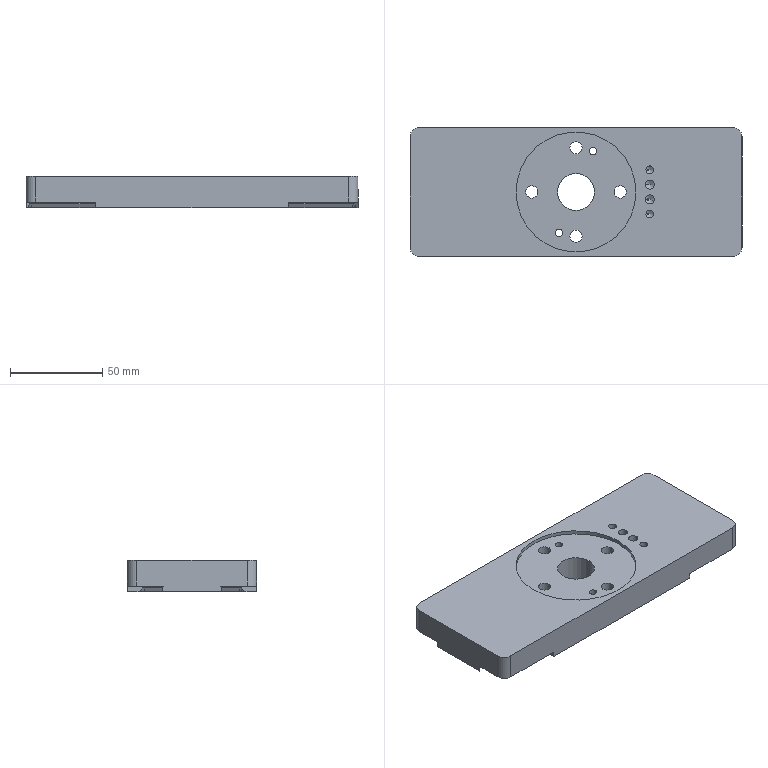Part | STEP file | 11-FG-E02411 | 1 solid | 139 faces | box 180 x 70 x 17 mm | volume 168926 mm3 | plane 59 | cylinder 56 | cone 24 | commonest cylinder face diameters 2 x16 6.6 x8 11 x8 3.3 x4 4 x4 4.2 x4